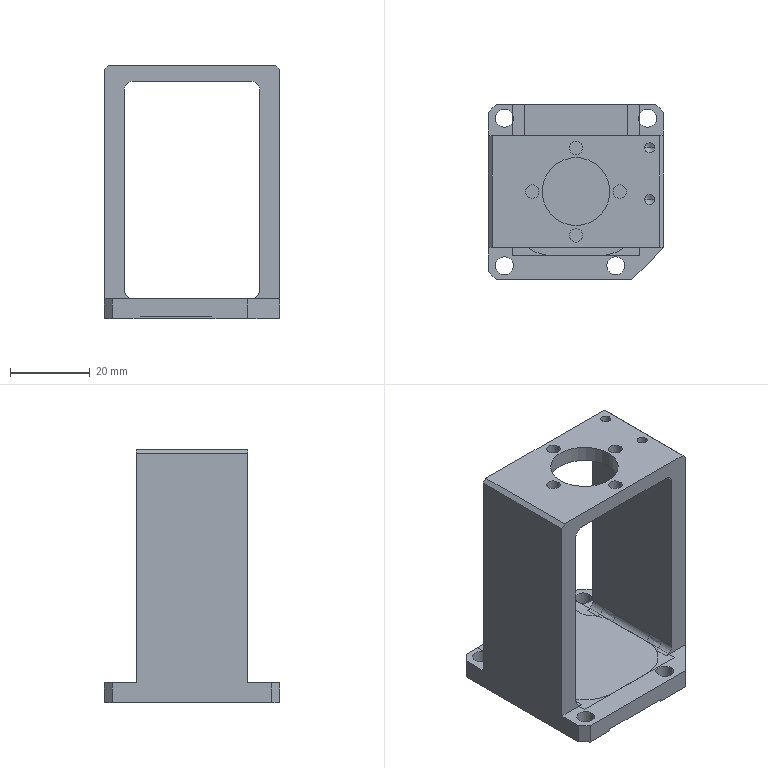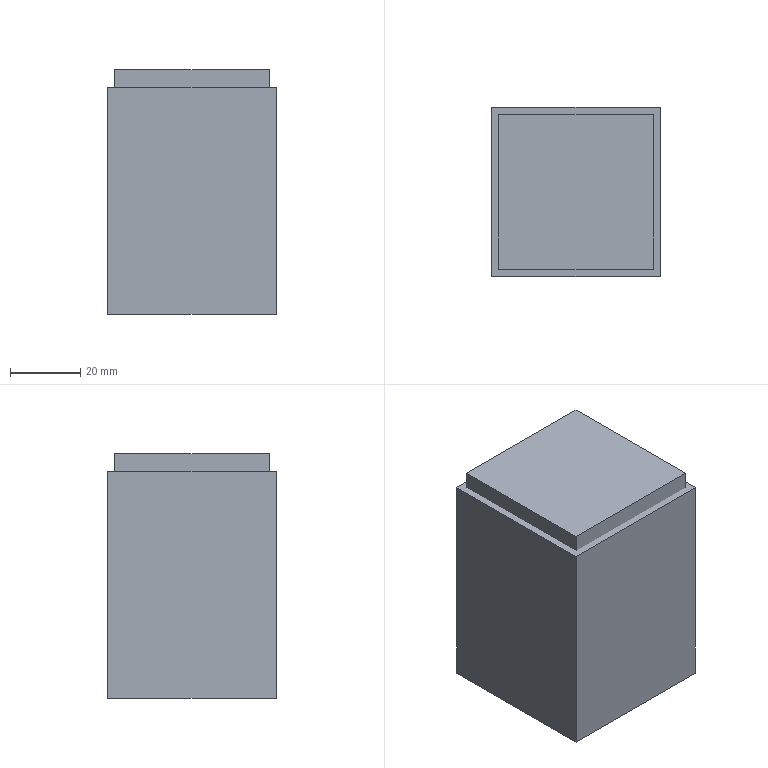CAM job | NX | 3+2 milling, drilling | part box 44 x 44 x 63.6 mm | stock box 48 x 48 x 69.6 mm
Tools:
number,name,description,diameter,corner_radius,flute_length,length,flutes
1,D63,Milling Tool-5 Parameters,63.0,0.0,50.0,75.0,2
7,D6A45,Milling Tool-5 Parameters,6.0,0.0,50.0,75.0,2
9,2.5ZT,Drilling Tool,2.5,0.0,35.0,50.0,2
8,3.4ZT,Drilling Tool,3.4,0.0,35.0,50.0,2
2,D20,Milling Tool-5 Parameters,20.0,0.0,50.0,75.0,2
13,D16JING,Milling Tool-5 Parameters,16.0,0.0,50.0,75.0,2
10,D10,Milling Tool-5 Parameters,10.0,0.0,50.0,75.0,2
11,D10JING,Milling Tool-5 Parameters,10.0,0.0,50.0,75.0,2
14,4.5ZT,Drilling Tool,4.5,0.0,35.0,50.0,2
4,D4,Milling Tool-5 Parameters,4.0,0.0,50.0,75.0,2
Operations:
program,operation,operation_type,tool,method,geometry_group,spindle_rpm,surface_speed,feed_per_tooth,feed_cut,feed_plunge,cut_length_mm,path_length_mm,cut_time_min,machine_time_min
1,FLOOR_WALL,VolumeBased25DMillingOperation,D63,METHOD,A,6500.0,1286.0,0.1154,1500.0,100.0,123.0,177.0,0.082,0.0874
1,DRILLING,Operation,D6A45,METHOD,A,5000.0,94.0,0.025,250.0,0.0,32.2,218.553,0.1288,0.1474
1,DRILLING_COPY,Operation,2.5ZT,METHOD,A,2000.0,10.0,0.02,80.0,0.0,22.502,121.346,0.2813,0.2912
1,DRILLING_COPY_COPY,Operation,3.4ZT,METHOD,A,2000.0,21.0,0.0375,150.0,0.0,38.086,192.701,0.2539,0.2694
1,ZLEVEL_PROFILE,ZLevelMilling,D20,METHOD,A,9500.0,298.0,0.1579,3000.0,1000.0,29669.844,29790.444,9.915,9.927
1,FLOOR_WALL_1,VolumeBased25DMillingOperation,D20,METHOD,A,9500.0,298.0,0.1316,2500.0,1000.0,15632.525,31094.689,6.666,8.212
1,FLOOR_WALL_1_COPY,VolumeBased25DMillingOperation,D16JING,METHOD,A,9500.0,298.0,0.0632,1200.0,1000.0,375.299,778.239,0.3145,0.3548
1,FLOOR_WALL_1_COPY_COPY,VolumeBased25DMillingOperation,D16JING,METHOD,A,9500.0,298.0,0.0632,1200.0,1000.0,762.535,1690.039,0.6414,0.7342
1,CAVITY_MILL_COPY_1,CavityMilling,D16JING,METHOD,A,9500.0,298.0,0.0632,1200.0,1000.0,1093.527,1475.994,0.9155,0.9537
1,HOLE_MILLING,CylinderMilling,D10,METHOD,A,9500.0,298.0,0.1053,2000.0,100.0,352.518,416.018,0.1763,0.1826
1,HOLE_MILLING_COPY_1_COPY,CylinderMilling,D10JING,METHOD,A,9500.0,298.0,0.0632,1200.0,100.0,53.154,116.654,0.0443,0.0506
1,PLANAR_MILL_COPY_1,PlanarMilling,D6A45,METHOD,A,9500.0,179.0,0.0658,1250.0,100.0,225.23,654.681,0.1802,0.2231
2,FLOOR_WALL_COPY,VolumeBased25DMillingOperation,D63,METHOD,B,6500.0,1286.0,0.1154,1500.0,100.0,738.0,1617.002,0.492,0.5799
2,FLOOR_WALL_1_COPY_1,VolumeBased25DMillingOperation,D10,METHOD,B,9500.0,298.0,0.1316,2500.0,1000.0,55.195,115.995,0.0237,0.0298
2,CAVITY_MILL,CavityMilling,D10,METHOD,B,9500.0,298.0,0.1316,2500.0,1000.0,2075.83,2653.532,0.9876,1.045
2,ZLEVEL_PROFILE_1,ZLevelMilling,D10JING,METHOD,B,9500.0,298.0,0.0658,1250.0,100.0,103.368,170.368,0.0827,0.0894
2,DRILLING_COPY_1,Operation,D6A45,METHOD,B,5000.0,94.0,0.025,250.0,0.0,18.4,232.606,0.0736,0.095
2,DRILLING_COPY_2,Operation,4.5ZT,METHOD,B,2000.0,28.0,0.0625,250.0,0.0,43.408,282.621,0.1736,0.1976
2,PLANAR_MILL_COPY_1_COPY,PlanarMilling,D6A45,METHOD,B,9500.0,179.0,0.0658,1250.0,100.0,278.678,780.903,0.2229,0.2732
2,PLANAR_MILL_COPY_1_COPY_COPY,PlanarMilling,D6A45,METHOD,B,9500.0,179.0,0.0658,1250.0,100.0,40.136,174.993,0.0321,0.0456
3,CAVITY_MILL_COPY,CavityMilling,D4,METHOD,C,9500.0,119.0,0.1053,2000.0,1000.0,71421.09,73191.978,36.876,37.053
3,CAVITY_MILL_COPY_COPY,CavityMilling,D4,METHOD,C,9500.0,119.0,0.0632,1200.0,1000.0,1001.934,1264.29,0.8378,0.8641
3,PLANAR_MILL_COPY_1_1_COPY_1,PlanarMilling,D6A45,METHOD,C,9500.0,179.0,0.0658,1250.0,100.0,138.367,213.367,0.1107,0.1182